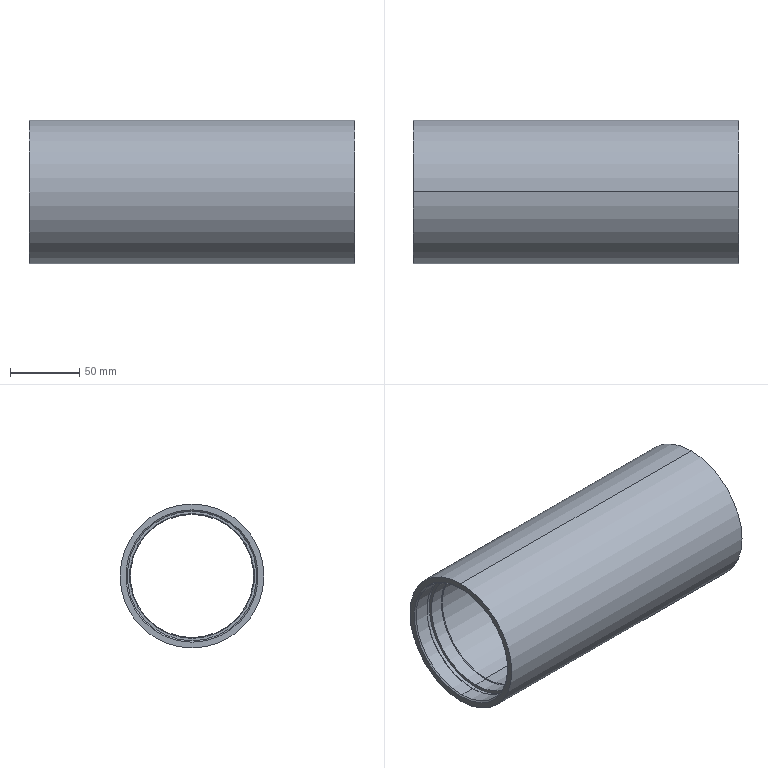Part | SolidWorks | features Chamfer 2, Revolution 1 | 1 solid | 30 faces | box 235 x 103.8 x 103.8 mm | volume 503241 mm3 | cylinder 16 | cone 8 | plane 6 | commonest cylinder face diameters 90 x4 93.5 x4 94.5 x4 89 x2 103.8 x2
STEP:
#1=CARTESIAN_POINT('',(25.5,0.,-44.5));
#2=VERTEX_POINT('',#1);
#3=CARTESIAN_POINT('',(25.5,0.,44.5));
#4=VERTEX_POINT('',#3);
#5=CARTESIAN_POINT('',(25.5,0.,0.));
#6=DIRECTION('',(-1.,0.,0.));
#7=DIRECTION('',(0.,0.,-1.));
#8=AXIS2_PLACEMENT_3D('',#5,#6,#7);
#9=CIRCLE('',#8,44.5);
#10=EDGE_CURVE('',#2,#4,#9,.T.);
#11=ORIENTED_EDGE('',*,*,#10,.F.);
#12=CARTESIAN_POINT('',(25.,0.,-45.));
#13=VERTEX_POINT('',#12);
#14=CARTESIAN_POINT('',(25.5,0.,-44.5));
#15=DIRECTION('',(-0.7071,0.,-0.7071));
#16=VECTOR('',#15,1000.);
#17=LINE('',#14,#16);
#18=EDGE_CURVE('',#2,#13,#17,.T.);
#19=ORIENTED_EDGE('',*,*,#18,.T.);
#20=CARTESIAN_POINT('',(25.,0.,45.));
#21=VERTEX_POINT('',#20);
#22=CARTESIAN_POINT('',(25.,0.,0.));
#23=DIRECTION('',(-1.,0.,0.));
#24=DIRECTION('',(0.,0.,1.));
#25=AXIS2_PLACEMENT_3D('',#22,#23,#24);
#26=CIRCLE('',#25,45.);
#27=EDGE_CURVE('',#13,#21,#26,.T.);
#28=ORIENTED_EDGE('',*,*,#27,.T.);
#29=CARTESIAN_POINT('',(25.5,0.,44.5));
#30=DIRECTION('',(-0.7071,0.,0.7071));
#31=VECTOR('',#30,1000.);
#32=LINE('',#29,#31);
#33=EDGE_CURVE('',#4,#21,#32,.T.);
#34=ORIENTED_EDGE('',*,*,#33,.F.);
#35=EDGE_LOOP('',(#11,#19,#28,#34));
#36=FACE_OUTER_BOUND('',#35,.T.);
#37=CARTESIAN_POINT('',(25.5,0.,0.));
#38=DIRECTION('',(-1.,0.,0.));
#39=DIRECTION('',(0.,0.,1.));
#40=AXIS2_PLACEMENT_3D('',#37,#38,#39);
#41=CONICAL_SURFACE('',#40,44.5,0.7854);
#42=ADVANCED_FACE('',(#36),#41,.F.);
#43=CARTESIAN_POINT('',(209.5,0.,44.5));
#44=VERTEX_POINT('',#43);
#45=CARTESIAN_POINT('',(209.5,0.,-44.5));
#46=VERTEX_POINT('',#45);
#47=CARTESIAN_POINT('',(209.5,0.,0.));
#48=DIRECTION('',(1.,0.,0.));
#49=DIRECTION('',(0.,0.,1.));
#50=AXIS2_PLACEMENT_3D('',#47,#48,#49);
#51=CIRCLE('',#50,44.5);
#52=EDGE_CURVE('',#44,#46,#51,.T.);
#53=ORIENTED_EDGE('',*,*,#52,.F.);
#54=CARTESIAN_POINT('',(210.,0.,45.));
#55=VERTEX_POINT('',#54);
#56=CARTESIAN_POINT('',(210.,0.,45.));
#57=DIRECTION('',(0.7071,0.,0.7071));
#58=VECTOR('',#57,1000.);
#59=LINE('',#56,#58);
#60=EDGE_CURVE('',#44,#55,#59,.T.);
#61=ORIENTED_EDGE('',*,*,#60,.T.);
#62=CARTESIAN_POINT('',(210.,0.,-45.));
#63=VERTEX_POINT('',#62);
#64=CARTESIAN_POINT('',(210.,0.,0.));
#65=DIRECTION('',(-1.,0.,0.));
#66=DIRECTION('',(0.,0.,1.));
#67=AXIS2_PLACEMENT_3D('',#64,#65,#66);
#68=CIRCLE('',#67,45.);
#69=EDGE_CURVE('',#63,#55,#68,.T.);
#70=ORIENTED_EDGE('',*,*,#69,.F.);
#71=CARTESIAN_POINT('',(210.,0.,-45.));
#72=DIRECTION('',(0.7071,0.,-0.7071));
#73=VECTOR('',#72,1000.);
#74=LINE('',#71,#73);
#75=EDGE_CURVE('',#46,#63,#74,.T.);
#76=ORIENTED_EDGE('',*,*,#75,.F.);
#77=EDGE_LOOP('',(#53,#61,#70,#76));
#78=FACE_OUTER_BOUND('',#77,.T.);
#79=CARTESIAN_POINT('',(210.,0.,0.));
#80=DIRECTION('',(1.,0.,0.));
#81=DIRECTION('',(0.,0.,-1.));
#82=AXIS2_PLACEMENT_3D('',#79,#80,#81);
#83=CONICAL_SURFACE('',#82,45.,0.7854);
#84=ADVANCED_FACE('',(#78),#83,.F.);
#85=CARTESIAN_POINT('',(1.,0.,-46.75));
#86=VERTEX_POINT('',#85);
#87=CARTESIAN_POINT('',(1.,0.,46.75));
#88=VERTEX_POINT('',#87);
#89=CARTESIAN_POINT('',(1.,0.,0.));
#90=DIRECTION('',(-1.,0.,0.));
#91=DIRECTION('',(0.,0.,-1.));
#92=AXIS2_PLACEMENT_3D('',#89,#90,#91);
#93=CIRCLE('',#92,46.75);
#94=EDGE_CURVE('',#86,#88,#93,.T.);
#95=ORIENTED_EDGE('',*,*,#94,.F.);
#96=CARTESIAN_POINT('',(0.,0.,-47.75));
#97=VERTEX_POINT('',#96);
#98=CARTESIAN_POINT('',(1.,0.,-46.75));
#99=DIRECTION('',(-0.7071,0.,-0.7071));
#100=VECTOR('',#99,1000.);
#101=LINE('',#98,#100);
#102=EDGE_CURVE('',#86,#97,#101,.T.);
#103=ORIENTED_EDGE('',*,*,#102,.T.);
#104=CARTESIAN_POINT('',(0.,0.,47.75));
#105=VERTEX_POINT('',#104);
#106=CARTESIAN_POINT('',(0.,0.,0.));
#107=DIRECTION('',(1.,0.,0.));
#108=DIRECTION('',(0.,0.,-1.));
#109=AXIS2_PLACEMENT_3D('',#106,#107,#108);
#110=CIRCLE('',#109,47.75);
#111=EDGE_CURVE('',#105,#97,#110,.T.);
#112=ORIENTED_EDGE('',*,*,#111,.F.);
#113=CARTESIAN_POINT('',(1.,0.,46.75));
#114=DIRECTION('',(-0.7071,0.,0.7071));
#115=VECTOR('',#114,1000.);
#116=LINE('',#113,#115);
#117=EDGE_CURVE('',#88,#105,#116,.T.);
#118=ORIENTED_EDGE('',*,*,#117,.F.);
#119=EDGE_LOOP('',(#95,#103,#112,#118));
#120=FACE_OUTER_BOUND('',#119,.T.);
#121=CARTESIAN_POINT('',(1.,0.,0.));
#122=DIRECTION('',(-1.,0.,0.));
#123=DIRECTION('',(0.,0.,1.));
#124=AXIS2_PLACEMENT_3D('',#121,#122,#123);
#125=CONICAL_SURFACE('',#124,46.75,0.7854);
#126=ADVANCED_FACE('',(#120),#125,.F.);
#127=CARTESIAN_POINT('',(234.,0.,46.75));
#128=VERTEX_POINT('',#127);
#129=CARTESIAN_POINT('',(234.,0.,-46.75));
#130=VERTEX_POINT('',#129);
#131=CARTESIAN_POINT('',(234.,0.,0.));
#132=DIRECTION('',(1.,0.,0.));
#133=DIRECTION('',(0.,0.,1.));
#134=AXIS2_PLACEMENT_3D('',#131,#132,#133);
#135=CIRCLE('',#134,46.75);
#136=EDGE_CURVE('',#128,#130,#135,.T.);
#137=ORIENTED_EDGE('',*,*,#136,.F.);
#138=CARTESIAN_POINT('',(235.,0.,47.75));
#139=VERTEX_POINT('',#138);
#140=CARTESIAN_POINT('',(235.,0.,47.75));
#141=DIRECTION('',(0.7071,0.,0.7071));
#142=VECTOR('',#141,1000.);
#143=LINE('',#140,#142);
#144=EDGE_CURVE('',#128,#139,#143,.T.);
#145=ORIENTED_EDGE('',*,*,#144,.T.);
#146=CARTESIAN_POINT('',(235.,0.,-47.75));
#147=VERTEX_POINT('',#146);
#148=CARTESIAN_POINT('',(235.,0.,0.));
#149=DIRECTION('',(-1.,0.,0.));
#150=DIRECTION('',(0.,0.,1.));
#151=AXIS2_PLACEMENT_3D('',#148,#149,#150);
#152=CIRCLE('',#151,47.75);
#153=EDGE_CURVE('',#147,#139,#152,.T.);
#154=ORIENTED_EDGE('',*,*,#153,.F.);
#155=CARTESIAN_POINT('',(235.,0.,-47.75));
#156=DIRECTION('',(0.7071,0.,-0.7071));
#157=VECTOR('',#156,1000.);
#158=LINE('',#155,#157);
#159=EDGE_CURVE('',#130,#147,#158,.T.);
#160=ORIENTED_EDGE('',*,*,#159,.F.);
#161=EDGE_LOOP('',(#137,#145,#154,#160));
#162=FACE_OUTER_BOUND('',#161,.T.);
#163=CARTESIAN_POINT('',(235.,0.,0.));
#164=DIRECTION('',(1.,0.,0.));
#165=DIRECTION('',(0.,0.,-1.));
#166=AXIS2_PLACEMENT_3D('',#163,#164,#165);
#167=CONICAL_SURFACE('',#166,47.75,0.7854);
#168=ADVANCED_FACE('',(#162),#167,.F.);
#169=CARTESIAN_POINT('',(12.,0.,-46.75));
#170=VERTEX_POINT('',#169);
#171=CARTESIAN_POINT('',(12.,0.,46.75));
#172=VERTEX_POINT('',#171);
#173=CARTESIAN_POINT('',(12.,0.,0.));
#174=DIRECTION('',(-1.,0.,0.));
#175=DIRECTION('',(0.,0.,1.));
#176=AXIS2_PLACEMENT_3D('',#173,#174,#175);
#177=CIRCLE('',#176,46.75);
#178=EDGE_CURVE('',#170,#172,#177,.T.);
#179=ORIENTED_EDGE('',*,*,#178,.F.);
#180=CARTESIAN_POINT('',(0.,0.,-46.75));
#181=DIRECTION('',(-1.,0.,0.));
#182=VECTOR('',#181,1000.);
#183=LINE('',#180,#182);
#184=EDGE_CURVE('',#170,#86,#183,.T.);
#185=ORIENTED_EDGE('',*,*,#184,.T.);
#186=ORIENTED_EDGE('',*,*,#94,.T.);
#187=CARTESIAN_POINT('',(0.,0.,46.75));
#188=DIRECTION('',(-1.,0.,0.));
#189=VECTOR('',#188,1000.);
#190=LINE('',#187,#189);
#191=EDGE_CURVE('',#172,#88,#190,.T.);
#192=ORIENTED_EDGE('',*,*,#191,.F.);
#193=EDGE_LOOP('',(#179,#185,#186,#192));
#194=FACE_OUTER_BOUND('',#193,.T.);
#195=CARTESIAN_POINT('',(0.,0.,0.));
#196=DIRECTION('',(-1.,0.,0.));
#197=DIRECTION('',(0.,0.,1.));
#198=AXIS2_PLACEMENT_3D('',#195,#196,#197);
#199=CYLINDRICAL_SURFACE('',#198,46.75);
#200=ADVANCED_FACE('',(#194),#199,.F.);
#201=CARTESIAN_POINT('',(15.,0.,-47.25));
#202=VERTEX_POINT('',#201);
#203=CARTESIAN_POINT('',(15.,0.,47.25));
#204=VERTEX_POINT('',#203);
#205=CARTESIAN_POINT('',(15.,0.,0.));
#206=DIRECTION('',(-1.,0.,0.));
#207=DIRECTION('',(0.,0.,1.));
#208=AXIS2_PLACEMENT_3D('',#205,#206,#207);
#209=CIRCLE('',#208,47.25);
#210=EDGE_CURVE('',#202,#204,#209,.T.);
#211=ORIENTED_EDGE('',*,*,#210,.F.);
#212=CARTESIAN_POINT('',(12.,0.,-47.25));
#213=VERTEX_POINT('',#212);
#214=CARTESIAN_POINT('',(0.,0.,-47.25));
#215=DIRECTION('',(-1.,0.,0.));
#216=VECTOR('',#215,1000.);
#217=LINE('',#214,#216);
#218=EDGE_CURVE('',#202,#213,#217,.T.);
#219=ORIENTED_EDGE('',*,*,#218,.T.);
#220=CARTESIAN_POINT('',(12.,0.,47.25));
#221=VERTEX_POINT('',#220);
#222=CARTESIAN_POINT('',(12.,0.,0.));
#223=DIRECTION('',(-1.,0.,0.));
#224=DIRECTION('',(0.,0.,1.));
#225=AXIS2_PLACEMENT_3D('',#222,#223,#224);
#226=CIRCLE('',#225,47.25);
#227=EDGE_CURVE('',#213,#221,#226,.T.);
#228=ORIENTED_EDGE('',*,*,#227,.T.);
#229=CARTESIAN_POINT('',(0.,0.,47.25));
#230=DIRECTION('',(-1.,0.,0.));
#231=VECTOR('',#230,1000.);
#232=LINE('',#229,#231);
#233=EDGE_CURVE('',#204,#221,#232,.T.);
#234=ORIENTED_EDGE('',*,*,#233,.F.);
#235=EDGE_LOOP('',(#211,#219,#228,#234));
#236=FACE_OUTER_BOUND('',#235,.T.);
#237=CARTESIAN_POINT('',(0.,0.,0.));
#238=DIRECTION('',(-1.,0.,0.));
#239=DIRECTION('',(0.,0.,1.));
#240=AXIS2_PLACEMENT_3D('',#237,#238,#239);
#241=CYLINDRICAL_SURFACE('',#240,47.25);
#242=ADVANCED_FACE('',(#236),#241,.F.);
#243=ORIENTED_EDGE('',*,*,#27,.F.);
#244=CARTESIAN_POINT('',(15.,0.,-45.));
#245=VERTEX_POINT('',#244);
#246=CARTESIAN_POINT('',(0.,0.,-45.));
#247=DIRECTION('',(-1.,0.,0.));
#248=VECTOR('',#247,1000.);
#249=LINE('',#246,#248);
#250=EDGE_CURVE('',#13,#245,#249,.T.);
#251=ORIENTED_EDGE('',*,*,#250,.T.);
#252=CARTESIAN_POINT('',(15.,0.,45.));
#253=VERTEX_POINT('',#252);
#254=CARTESIAN_POINT('',(15.,0.,0.));
#255=DIRECTION('',(-1.,0.,0.));
#256=DIRECTION('',(0.,0.,1.));
#257=AXIS2_PLACEMENT_3D('',#254,#255,#256);
#258=CIRCLE('',#257,45.);
#259=EDGE_CURVE('',#245,#253,#258,.T.);
#260=ORIENTED_EDGE('',*,*,#259,.T.);
#261=CARTESIAN_POINT('',(0.,0.,45.));
#262=DIRECTION('',(-1.,0.,0.));
#263=VECTOR('',#262,1000.);
#264=LINE('',#261,#263);
#265=EDGE_CURVE('',#21,#253,#264,.T.);
#266=ORIENTED_EDGE('',*,*,#265,.F.);
#267=EDGE_LOOP('',(#243,#251,#260,#266));
#268=FACE_OUTER_BOUND('',#267,.T.);
#269=CARTESIAN_POINT('',(0.,0.,0.));
#270=DIRECTION('',(-1.,0.,0.));
#271=DIRECTION('',(0.,0.,1.));
#272=AXIS2_PLACEMENT_3D('',#269,#270,#271);
#273=CYLINDRICAL_SURFACE('',#272,45.);
#274=ADVANCED_FACE('',(#268),#273,.F.);
#275=ORIENTED_EDGE('',*,*,#52,.T.);
#276=CARTESIAN_POINT('',(0.,0.,-44.5));
#277=DIRECTION('',(-1.,0.,0.));
#278=VECTOR('',#277,1000.);
#279=LINE('',#276,#278);
#280=EDGE_CURVE('',#46,#2,#279,.T.);
#281=ORIENTED_EDGE('',*,*,#280,.T.);
#282=ORIENTED_EDGE('',*,*,#10,.T.);
#283=CARTESIAN_POINT('',(0.,0.,44.5));
#284=DIRECTION('',(-1.,0.,0.));
#285=VECTOR('',#284,1000.);
#286=LINE('',#283,#285);
#287=EDGE_CURVE('',#44,#4,#286,.T.);
#288=ORIENTED_EDGE('',*,*,#287,.F.);
#289=EDGE_LOOP('',(#275,#281,#282,#288));
#290=FACE_OUTER_BOUND('',#289,.T.);
#291=CARTESIAN_POINT('',(0.,0.,0.));
#292=DIRECTION('',(-1.,0.,0.));
#293=DIRECTION('',(0.,0.,1.));
#294=AXIS2_PLACEMENT_3D('',#291,#292,#293);
#295=CYLINDRICAL_SURFACE('',#294,44.5);
#296=ADVANCED_FACE('',(#290),#295,.F.);
#297=CARTESIAN_POINT('',(220.,0.,-45.));
#298=VERTEX_POINT('',#297);
#299=CARTESIAN_POINT('',(220.,0.,45.));
#300=VERTEX_POINT('',#299);
#301=CARTESIAN_POINT('',(220.,0.,0.));
#302=DIRECTION('',(-1.,0.,0.));
#303=DIRECTION('',(0.,0.,1.));
#304=AXIS2_PLACEMENT_3D('',#301,#302,#303);
#305=CIRCLE('',#304,45.);
#306=EDGE_CURVE('',#298,#300,#305,.T.);
#307=ORIENTED_EDGE('',*,*,#306,.F.);
#308=CARTESIAN_POINT('',(0.,0.,-45.));
#309=DIRECTION('',(-1.,0.,0.));
#310=VECTOR('',#309,1000.);
#311=LINE('',#308,#310);
#312=EDGE_CURVE('',#298,#63,#311,.T.);
#313=ORIENTED_EDGE('',*,*,#312,.T.);
#314=ORIENTED_EDGE('',*,*,#69,.T.);
#315=CARTESIAN_POINT('',(0.,0.,45.));
#316=DIRECTION('',(-1.,0.,0.));
#317=VECTOR('',#316,1000.);
#318=LINE('',#315,#317);
#319=EDGE_CURVE('',#300,#55,#318,.T.);
#320=ORIENTED_EDGE('',*,*,#319,.F.);
#321=EDGE_LOOP('',(#307,#313,#314,#320));
#322=FACE_OUTER_BOUND('',#321,.T.);
#323=CARTESIAN_POINT('',(0.,0.,0.));
#324=DIRECTION('',(-1.,0.,0.));
#325=DIRECTION('',(0.,0.,1.));
#326=AXIS2_PLACEMENT_3D('',#323,#324,#325);
#327=CYLINDRICAL_SURFACE('',#326,45.);
#328=ADVANCED_FACE('',(#322),#327,.F.);
#329=CARTESIAN_POINT('',(223.,0.,-47.25));
#330=VERTEX_POINT('',#329);
#331=CARTESIAN_POINT('',(223.,0.,47.25));
#332=VERTEX_POINT('',#331);
#333=CARTESIAN_POINT('',(223.,0.,0.));
#334=DIRECTION('',(-1.,0.,0.));
#335=DIRECTION('',(0.,0.,1.));
#336=AXIS2_PLACEMENT_3D('',#333,#334,#335);
#337=CIRCLE('',#336,47.25);
#338=EDGE_CURVE('',#330,#332,#337,.T.);
#339=ORIENTED_EDGE('',*,*,#338,.F.);
#340=CARTESIAN_POINT('',(220.,0.,-47.25));
#341=VERTEX_POINT('',#340);
#342=CARTESIAN_POINT('',(0.,0.,-47.25));
#343=DIRECTION('',(-1.,0.,0.));
#344=VECTOR('',#343,1000.);
#345=LINE('',#342,#344);
#346=EDGE_CURVE('',#330,#341,#345,.T.);
#347=ORIENTED_EDGE('',*,*,#346,.T.);
#348=CARTESIAN_POINT('',(220.,0.,47.25));
#349=VERTEX_POINT('',#348);
#350=CARTESIAN_POINT('',(220.,0.,0.));
#351=DIRECTION('',(-1.,0.,0.));
#352=DIRECTION('',(0.,0.,1.));
#353=AXIS2_PLACEMENT_3D('',#350,#351,#352);
#354=CIRCLE('',#353,47.25);
#355=EDGE_CURVE('',#341,#349,#354,.T.);
#356=ORIENTED_EDGE('',*,*,#355,.T.);
#357=CARTESIAN_POINT('',(0.,0.,47.25));
#358=DIRECTION('',(-1.,0.,0.));
#359=VECTOR('',#358,1000.);
#360=LINE('',#357,#359);
#361=EDGE_CURVE('',#332,#349,#360,.T.);
#362=ORIENTED_EDGE('',*,*,#361,.F.);
#363=EDGE_LOOP('',(#339,#347,#356,#362));
#364=FACE_OUTER_BOUND('',#363,.T.);
#365=CARTESIAN_POINT('',(0.,0.,0.));
#366=DIRECTION('',(-1.,0.,0.));
#367=DIRECTION('',(0.,0.,1.));
#368=AXIS2_PLACEMENT_3D('',#365,#366,#367);
#369=CYLINDRICAL_SURFACE('',#368,47.25);
#370=ADVANCED_FACE('',(#364),#369,.F.);
#371=ORIENTED_EDGE('',*,*,#136,.T.);
#372=CARTESIAN_POINT('',(223.,0.,-46.75));
#373=VERTEX_POINT('',#372);
#374=CARTESIAN_POINT('',(0.,0.,-46.75));
#375=DIRECTION('',(-1.,0.,0.));
#376=VECTOR('',#375,1000.);
#377=LINE('',#374,#376);
#378=EDGE_CURVE('',#130,#373,#377,.T.);
#379=ORIENTED_EDGE('',*,*,#378,.T.);
#380=CARTESIAN_POINT('',(223.,0.,46.75));
#381=VERTEX_POINT('',#380);
#382=CARTESIAN_POINT('',(223.,0.,0.));
#383=DIRECTION('',(-1.,0.,0.));
#384=DIRECTION('',(0.,0.,1.));
#385=AXIS2_PLACEMENT_3D('',#382,#383,#384);
#386=CIRCLE('',#385,46.75);
#387=EDGE_CURVE('',#373,#381,#386,.T.);
#388=ORIENTED_EDGE('',*,*,#387,.T.);
#389=CARTESIAN_POINT('',(0.,0.,46.75));
#390=DIRECTION('',(-1.,0.,0.));
#391=VECTOR('',#390,1000.);
#392=LINE('',#389,#391);
#393=EDGE_CURVE('',#128,#381,#392,.T.);
#394=ORIENTED_EDGE('',*,*,#393,.F.);
#395=EDGE_LOOP('',(#371,#379,#388,#394));
#396=FACE_OUTER_BOUND('',#395,.T.);
#397=CARTESIAN_POINT('',(0.,0.,0.));
#398=DIRECTION('',(-1.,0.,0.));
#399=DIRECTION('',(0.,0.,1.));
#400=AXIS2_PLACEMENT_3D('',#397,#398,#399);
#401=CYLINDRICAL_SURFACE('',#400,46.75);
#402=ADVANCED_FACE('',(#396),#401,.F.);
#403=CARTESIAN_POINT('',(235.,0.,51.9));
#404=VERTEX_POINT('',#403);
#405=CARTESIAN_POINT('',(235.,0.,-51.9));
#406=VERTEX_POINT('',#405);
#407=CARTESIAN_POINT('',(235.,0.,0.));
#408=DIRECTION('',(-1.,0.,0.));
#409=DIRECTION('',(0.,0.,1.));
#410=AXIS2_PLACEMENT_3D('',#407,#408,#409);
#411=CIRCLE('',#410,51.9);
#412=EDGE_CURVE('',#404,#406,#411,.T.);
#413=ORIENTED_EDGE('',*,*,#412,.T.);
#414=CARTESIAN_POINT('',(0.,0.,-51.9));
#415=VERTEX_POINT('',#414);
#416=CARTESIAN_POINT('',(0.,0.,-51.9));
#417=DIRECTION('',(-1.,0.,0.));
#418=VECTOR('',#417,1000.);
#419=LINE('',#416,#418);
#420=EDGE_CURVE('',#406,#415,#419,.T.);
#421=ORIENTED_EDGE('',*,*,#420,.T.);
#422=CARTESIAN_POINT('',(0.,0.,51.9));
#423=VERTEX_POINT('',#422);
#424=CARTESIAN_POINT('',(0.,0.,0.));
#425=DIRECTION('',(-1.,0.,0.));
#426=DIRECTION('',(0.,0.,1.));
#427=AXIS2_PLACEMENT_3D('',#424,#425,#426);
#428=CIRCLE('',#427,51.9);
#429=EDGE_CURVE('',#423,#415,#428,.T.);
#430=ORIENTED_EDGE('',*,*,#429,.F.);
#431=CARTESIAN_POINT('',(0.,0.,51.9));
#432=DIRECTION('',(-1.,0.,0.));
#433=VECTOR('',#432,1000.);
#434=LINE('',#431,#433);
#435=EDGE_CURVE('',#404,#423,#434,.T.);
#436=ORIENTED_EDGE('',*,*,#435,.F.);
#437=EDGE_LOOP('',(#413,#421,#430,#436));
#438=FACE_OUTER_BOUND('',#437,.T.);
#439=CARTESIAN_POINT('',(0.,0.,0.));
#440=DIRECTION('',(-1.,0.,0.));
#441=DIRECTION('',(0.,0.,1.));
#442=AXIS2_PLACEMENT_3D('',#439,#440,#441);
#443=CYLINDRICAL_SURFACE('',#442,51.9);
#444=ADVANCED_FACE('',(#438),#443,.T.);
#445=ORIENTED_EDGE('',*,*,#111,.T.);
#446=CARTESIAN_POINT('',(0.,0.,0.));
#447=DIRECTION('',(1.,0.,0.));
#448=DIRECTION('',(0.,0.,-1.));
#449=AXIS2_PLACEMENT_3D('',#446,#447,#448);
#450=CIRCLE('',#449,47.75);
#451=EDGE_CURVE('',#97,#105,#450,.T.);
#452=ORIENTED_EDGE('',*,*,#451,.T.);
#453=EDGE_LOOP('',(#445,#452));
#454=FACE_BOUND('',#453,.T.);
#455=ORIENTED_EDGE('',*,*,#429,.T.);
#456=CARTESIAN_POINT('',(0.,0.,0.));
#457=DIRECTION('',(-1.,0.,0.));
#458=DIRECTION('',(0.,0.,1.));
#459=AXIS2_PLACEMENT_3D('',#456,#457,#458);
#460=CIRCLE('',#459,51.9);
#461=EDGE_CURVE('',#415,#423,#460,.T.);
#462=ORIENTED_EDGE('',*,*,#461,.T.);
#463=EDGE_LOOP('',(#455,#462));
#464=FACE_OUTER_BOUND('',#463,.T.);
#465=CARTESIAN_POINT('',(0.,0.,-46.75));
#466=DIRECTION('',(1.,0.,0.));
#467=DIRECTION('',(0.,0.,-1.));
#468=AXIS2_PLACEMENT_3D('',#465,#466,#467);
#469=PLANE('',#468);
#470=ADVANCED_FACE('',(#454,#464),#469,.F.);
#471=ORIENTED_EDGE('',*,*,#420,.F.);
#472=CARTESIAN_POINT('',(235.,0.,0.));
#473=DIRECTION('',(-1.,0.,0.));
#474=DIRECTION('',(0.,0.,1.));
#475=AXIS2_PLACEMENT_3D('',#472,#473,#474);
#476=CIRCLE('',#475,51.9);
#477=EDGE_CURVE('',#406,#404,#476,.T.);
#478=ORIENTED_EDGE('',*,*,#477,.T.);
#479=ORIENTED_EDGE('',*,*,#435,.T.);
#480=ORIENTED_EDGE('',*,*,#461,.F.);
#481=EDGE_LOOP('',(#471,#478,#479,#480));
#482=FACE_OUTER_BOUND('',#481,.T.);
#483=CARTESIAN_POINT('',(0.,0.,0.));
#484=DIRECTION('',(-1.,0.,0.));
#485=DIRECTION('',(0.,0.,1.));
#486=AXIS2_PLACEMENT_3D('',#483,#484,#485);
#487=CYLINDRICAL_SURFACE('',#486,51.9);
#488=ADVANCED_FACE('',(#482),#487,.T.);
#489=ORIENTED_EDGE('',*,*,#153,.T.);
#490=CARTESIAN_POINT('',(235.,0.,0.));
#491=DIRECTION('',(-1.,0.,0.));
#492=DIRECTION('',(0.,0.,1.));
#493=AXIS2_PLACEMENT_3D('',#490,#491,#492);
#494=CIRCLE('',#493,47.75);
#495=EDGE_CURVE('',#139,#147,#494,.T.);
#496=ORIENTED_EDGE('',*,*,#495,.T.);
#497=EDGE_LOOP('',(#489,#496));
#498=FACE_BOUND('',#497,.T.);
#499=ORIENTED_EDGE('',*,*,#412,.F.);
#500=ORIENTED_EDGE('',*,*,#477,.F.);
#501=EDGE_LOOP('',(#499,#500));
#502=FACE_OUTER_BOUND('',#501,.T.);
#503=CARTESIAN_POINT('',(235.,0.,-46.75));
#504=DIRECTION('',(-1.,0.,0.));
#505=DIRECTION('',(0.,0.,1.));
#506=AXIS2_PLACEMENT_3D('',#503,#504,#505);
#507=PLANE('',#506);
#508=ADVANCED_FACE('',(#498,#502),#507,.F.);
#509=ORIENTED_EDGE('',*,*,#378,.F.);
#510=CARTESIAN_POINT('',(234.,0.,0.));
#511=DIRECTION('',(1.,0.,0.));
#512=DIRECTION('',(0.,0.,1.));
#513=AXIS2_PLACEMENT_3D('',#510,#511,#512);
#514=CIRCLE('',#513,46.75);
#515=EDGE_CURVE('',#130,#128,#514,.T.);
#516=ORIENTED_EDGE('',*,*,#515,.T.);
#517=ORIENTED_EDGE('',*,*,#393,.T.);
#518=CARTESIAN_POINT('',(223.,0.,0.));
#519=DIRECTION('',(-1.,0.,0.));
#520=DIRECTION('',(0.,0.,1.));
#521=AXIS2_PLACEMENT_3D('',#518,#519,#520);
#522=CIRCLE('',#521,46.75);
#523=EDGE_CURVE('',#381,#373,#522,.T.);
#524=ORIENTED_EDGE('',*,*,#523,.T.);
#525=EDGE_LOOP('',(#509,#516,#517,#524));
#526=FACE_OUTER_BOUND('',#525,.T.);
#527=CARTESIAN_POINT('',(0.,0.,0.));
#528=DIRECTION('',(-1.,0.,0.));
#529=DIRECTION('',(0.,0.,1.));
#530=AXIS2_PLACEMENT_3D('',#527,#528,#529);
#531=CYLINDRICAL_SURFACE('',#530,46.75);
#532=ADVANCED_FACE('',(#526),#531,.F.);
#533=ORIENTED_EDGE('',*,*,#523,.F.);
#534=ORIENTED_EDGE('',*,*,#387,.F.);
#535=EDGE_LOOP('',(#533,#534));
#536=FACE_BOUND('',#535,.T.);
#537=CARTESIAN_POINT('',(223.,0.,0.));
#538=DIRECTION('',(-1.,0.,0.));
#539=DIRECTION('',(0.,0.,1.));
#540=AXIS2_PLACEMENT_3D('',#537,#538,#539);
#541=CIRCLE('',#540,47.25);
#542=EDGE_CURVE('',#332,#330,#541,.T.);
#543=ORIENTED_EDGE('',*,*,#542,.T.);
#544=ORIENTED_EDGE('',*,*,#338,.T.);
#545=EDGE_LOOP('',(#543,#544));
#546=FACE_OUTER_BOUND('',#545,.T.);
#547=CARTESIAN_POINT('',(223.,0.,-46.75));
#548=DIRECTION('',(1.,0.,0.));
#549=DIRECTION('',(0.,0.,-1.));
#550=AXIS2_PLACEMENT_3D('',#547,#548,#549);
#551=PLANE('',#550);
#552=ADVANCED_FACE('',(#536,#546),#551,.F.);
#553=ORIENTED_EDGE('',*,*,#346,.F.);
#554=ORIENTED_EDGE('',*,*,#542,.F.);
#555=ORIENTED_EDGE('',*,*,#361,.T.);
#556=CARTESIAN_POINT('',(220.,0.,0.));
#557=DIRECTION('',(-1.,0.,0.));
#558=DIRECTION('',(0.,0.,1.));
#559=AXIS2_PLACEMENT_3D('',#556,#557,#558);
#560=CIRCLE('',#559,47.25);
#561=EDGE_CURVE('',#349,#341,#560,.T.);
#562=ORIENTED_EDGE('',*,*,#561,.T.);
#563=EDGE_LOOP('',(#553,#554,#555,#562));
#564=FACE_OUTER_BOUND('',#563,.T.);
#565=CARTESIAN_POINT('',(0.,0.,0.));
#566=DIRECTION('',(-1.,0.,0.));
#567=DIRECTION('',(0.,0.,1.));
#568=AXIS2_PLACEMENT_3D('',#565,#566,#567);
#569=CYLINDRICAL_SURFACE('',#568,47.25);
#570=ADVANCED_FACE('',(#564),#569,.F.);
#571=ORIENTED_EDGE('',*,*,#561,.F.);
#572=ORIENTED_EDGE('',*,*,#355,.F.);
#573=EDGE_LOOP('',(#571,#572));
#574=FACE_OUTER_BOUND('',#573,.T.);
#575=CARTESIAN_POINT('',(220.,0.,0.));
#576=DIRECTION('',(-1.,0.,0.));
#577=DIRECTION('',(0.,0.,1.));
#578=AXIS2_PLACEMENT_3D('',#575,#576,#577);
#579=CIRCLE('',#578,45.);
#580=EDGE_CURVE('',#300,#298,#579,.T.);
#581=ORIENTED_EDGE('',*,*,#580,.T.);
#582=ORIENTED_EDGE('',*,*,#306,.T.);
#583=EDGE_LOOP('',(#581,#582));
#584=FACE_BOUND('',#583,.T.);
#585=CARTESIAN_POINT('',(220.,0.,-47.25));
#586=DIRECTION('',(-1.,0.,0.));
#587=DIRECTION('',(0.,0.,1.));
#588=AXIS2_PLACEMENT_3D('',#585,#586,#587);
#589=PLANE('',#588);
#590=ADVANCED_FACE('',(#574,#584),#589,.F.);
#591=ORIENTED_EDGE('',*,*,#312,.F.);
#592=ORIENTED_EDGE('',*,*,#580,.F.);
#593=ORIENTED_EDGE('',*,*,#319,.T.);
#594=CARTESIAN_POINT('',(210.,0.,0.));
#595=DIRECTION('',(-1.,0.,0.));
#596=DIRECTION('',(0.,0.,1.));
#597=AXIS2_PLACEMENT_3D('',#594,#595,#596);
#598=CIRCLE('',#597,45.);
#599=EDGE_CURVE('',#55,#63,#598,.T.);
#600=ORIENTED_EDGE('',*,*,#599,.T.);
#601=EDGE_LOOP('',(#591,#592,#593,#600));
#602=FACE_OUTER_BOUND('',#601,.T.);
#603=CARTESIAN_POINT('',(0.,0.,0.));
#604=DIRECTION('',(-1.,0.,0.));
#605=DIRECTION('',(0.,0.,1.));
#606=AXIS2_PLACEMENT_3D('',#603,#604,#605);
#607=CYLINDRICAL_SURFACE('',#606,45.);
#608=ADVANCED_FACE('',(#602),#607,.F.);
#609=ORIENTED_EDGE('',*,*,#280,.F.);
#610=CARTESIAN_POINT('',(209.5,0.,0.));
#611=DIRECTION('',(1.,0.,0.));
#612=DIRECTION('',(0.,0.,1.));
#613=AXIS2_PLACEMENT_3D('',#610,#611,#612);
#614=CIRCLE('',#613,44.5);
#615=EDGE_CURVE('',#46,#44,#614,.T.);
#616=ORIENTED_EDGE('',*,*,#615,.T.);
#617=ORIENTED_EDGE('',*,*,#287,.T.);
#618=CARTESIAN_POINT('',(25.5,0.,0.));
#619=DIRECTION('',(-1.,0.,0.));
#620=DIRECTION('',(0.,0.,-1.));
#621=AXIS2_PLACEMENT_3D('',#618,#619,#620);
#622=CIRCLE('',#621,44.5);
#623=EDGE_CURVE('',#4,#2,#622,.T.);
#624=ORIENTED_EDGE('',*,*,#623,.T.);
#625=EDGE_LOOP('',(#609,#616,#617,#624));
#626=FACE_OUTER_BOUND('',#625,.T.);
#627=CARTESIAN_POINT('',(0.,0.,0.));
#628=DIRECTION('',(-1.,0.,0.));
#629=DIRECTION('',(0.,0.,1.));
#630=AXIS2_PLACEMENT_3D('',#627,#628,#629);
#631=CYLINDRICAL_SURFACE('',#630,44.5);
#632=ADVANCED_FACE('',(#626),#631,.F.);
#633=ORIENTED_EDGE('',*,*,#250,.F.);
#634=CARTESIAN_POINT('',(25.,0.,0.));
#635=DIRECTION('',(-1.,0.,0.));
#636=DIRECTION('',(0.,0.,1.));
#637=AXIS2_PLACEMENT_3D('',#634,#635,#636);
#638=CIRCLE('',#637,45.);
#639=EDGE_CURVE('',#21,#13,#638,.T.);
#640=ORIENTED_EDGE('',*,*,#639,.F.);
#641=ORIENTED_EDGE('',*,*,#265,.T.);
#642=CARTESIAN_POINT('',(15.,0.,0.));
#643=DIRECTION('',(-1.,0.,0.));
#644=DIRECTION('',(0.,0.,1.));
#645=AXIS2_PLACEMENT_3D('',#642,#643,#644);
#646=CIRCLE('',#645,45.);
#647=EDGE_CURVE('',#253,#245,#646,.T.);
#648=ORIENTED_EDGE('',*,*,#647,.T.);
#649=EDGE_LOOP('',(#633,#640,#641,#648));
#650=FACE_OUTER_BOUND('',#649,.T.);
#651=CARTESIAN_POINT('',(0.,0.,0.));
#652=DIRECTION('',(-1.,0.,0.));
#653=DIRECTION('',(0.,0.,1.));
#654=AXIS2_PLACEMENT_3D('',#651,#652,#653);
#655=CYLINDRICAL_SURFACE('',#654,45.);
#656=ADVANCED_FACE('',(#650),#655,.F.);
#657=ORIENTED_EDGE('',*,*,#647,.F.);
#658=ORIENTED_EDGE('',*,*,#259,.F.);
#659=EDGE_LOOP('',(#657,#658));
#660=FACE_BOUND('',#659,.T.);
#661=CARTESIAN_POINT('',(15.,0.,0.));
#662=DIRECTION('',(-1.,0.,0.));
#663=DIRECTION('',(0.,0.,1.));
#664=AXIS2_PLACEMENT_3D('',#661,#662,#663);
#665=CIRCLE('',#664,47.25);
#666=EDGE_CURVE('',#204,#202,#665,.T.);
#667=ORIENTED_EDGE('',*,*,#666,.T.);
#668=ORIENTED_EDGE('',*,*,#210,.T.);
#669=EDGE_LOOP('',(#667,#668));
#670=FACE_OUTER_BOUND('',#669,.T.);
#671=CARTESIAN_POINT('',(15.,0.,-47.25));
#672=DIRECTION('',(1.,0.,0.));
#673=DIRECTION('',(0.,0.,-1.));
#674=AXIS2_PLACEMENT_3D('',#671,#672,#673);
#675=PLANE('',#674);
#676=ADVANCED_FACE('',(#660,#670),#675,.F.);
#677=ORIENTED_EDGE('',*,*,#218,.F.);
#678=ORIENTED_EDGE('',*,*,#666,.F.);
#679=ORIENTED_EDGE('',*,*,#233,.T.);
#680=CARTESIAN_POINT('',(12.,0.,0.));
#681=DIRECTION('',(-1.,0.,0.));
#682=DIRECTION('',(0.,0.,1.));
#683=AXIS2_PLACEMENT_3D('',#680,#681,#682);
#684=CIRCLE('',#683,47.25);
#685=EDGE_CURVE('',#221,#213,#684,.T.);
#686=ORIENTED_EDGE('',*,*,#685,.T.);
#687=EDGE_LOOP('',(#677,#678,#679,#686));
#688=FACE_OUTER_BOUND('',#687,.T.);
#689=CARTESIAN_POINT('',(0.,0.,0.));
#690=DIRECTION('',(-1.,0.,0.));
#691=DIRECTION('',(0.,0.,1.));
#692=AXIS2_PLACEMENT_3D('',#689,#690,#691);
#693=CYLINDRICAL_SURFACE('',#692,47.25);
#694=ADVANCED_FACE('',(#688),#693,.F.);
#695=ORIENTED_EDGE('',*,*,#685,.F.);
#696=ORIENTED_EDGE('',*,*,#227,.F.);
#697=EDGE_LOOP('',(#695,#696));
#698=FACE_OUTER_BOUND('',#697,.T.);
#699=CARTESIAN_POINT('',(12.,0.,0.));
#700=DIRECTION('',(-1.,0.,0.));
#701=DIRECTION('',(0.,0.,1.));
#702=AXIS2_PLACEMENT_3D('',#699,#700,#701);
#703=CIRCLE('',#702,46.75);
#704=EDGE_CURVE('',#172,#170,#703,.T.);
#705=ORIENTED_EDGE('',*,*,#704,.T.);
#706=ORIENTED_EDGE('',*,*,#178,.T.);
#707=EDGE_LOOP('',(#705,#706));
#708=FACE_BOUND('',#707,.T.);
#709=CARTESIAN_POINT('',(12.,0.,-46.75));
#710=DIRECTION('',(-1.,0.,0.));
#711=DIRECTION('',(0.,0.,1.));
#712=AXIS2_PLACEMENT_3D('',#709,#710,#711);
#713=PLANE('',#712);
#714=ADVANCED_FACE('',(#698,#708),#713,.F.);
#715=ORIENTED_EDGE('',*,*,#184,.F.);
#716=ORIENTED_EDGE('',*,*,#704,.F.);
#717=ORIENTED_EDGE('',*,*,#191,.T.);
#718=CARTESIAN_POINT('',(1.,0.,0.));
#719=DIRECTION('',(-1.,0.,0.));
#720=DIRECTION('',(0.,0.,-1.));
#721=AXIS2_PLACEMENT_3D('',#718,#719,#720);
#722=CIRCLE('',#721,46.75);
#723=EDGE_CURVE('',#88,#86,#722,.T.);
#724=ORIENTED_EDGE('',*,*,#723,.T.);
#725=EDGE_LOOP('',(#715,#716,#717,#724));
#726=FACE_OUTER_BOUND('',#725,.T.);
#727=CARTESIAN_POINT('',(0.,0.,0.));
#728=DIRECTION('',(-1.,0.,0.));
#729=DIRECTION('',(0.,0.,1.));
#730=AXIS2_PLACEMENT_3D('',#727,#728,#729);
#731=CYLINDRICAL_SURFACE('',#730,46.75);
#732=ADVANCED_FACE('',(#726),#731,.F.);
#733=ORIENTED_EDGE('',*,*,#144,.F.);
#734=ORIENTED_EDGE('',*,*,#515,.F.);
#735=ORIENTED_EDGE('',*,*,#159,.T.);
#736=ORIENTED_EDGE('',*,*,#495,.F.);
#737=EDGE_LOOP('',(#733,#734,#735,#736));
#738=FACE_OUTER_BOUND('',#737,.T.);
#739=CARTESIAN_POINT('',(235.,0.,0.));
#740=DIRECTION('',(1.,0.,0.));
#741=DIRECTION('',(0.,0.,-1.));
#742=AXIS2_PLACEMENT_3D('',#739,#740,#741);
#743=CONICAL_SURFACE('',#742,47.75,0.7854);
#744=ADVANCED_FACE('',(#738),#743,.F.);
#745=ORIENTED_EDGE('',*,*,#102,.F.);
#746=ORIENTED_EDGE('',*,*,#723,.F.);
#747=ORIENTED_EDGE('',*,*,#117,.T.);
#748=ORIENTED_EDGE('',*,*,#451,.F.);
#749=EDGE_LOOP('',(#745,#746,#747,#748));
#750=FACE_OUTER_BOUND('',#749,.T.);
#751=CARTESIAN_POINT('',(1.,0.,0.));
#752=DIRECTION('',(-1.,0.,0.));
#753=DIRECTION('',(0.,0.,1.));
#754=AXIS2_PLACEMENT_3D('',#751,#752,#753);
#755=CONICAL_SURFACE('',#754,46.75,0.7854);
#756=ADVANCED_FACE('',(#750),#755,.F.);
#757=ORIENTED_EDGE('',*,*,#60,.F.);
#758=ORIENTED_EDGE('',*,*,#615,.F.);
#759=ORIENTED_EDGE('',*,*,#75,.T.);
#760=ORIENTED_EDGE('',*,*,#599,.F.);
#761=EDGE_LOOP('',(#757,#758,#759,#760));
#762=FACE_OUTER_BOUND('',#761,.T.);
#763=CARTESIAN_POINT('',(210.,0.,0.));
#764=DIRECTION('',(1.,0.,0.));
#765=DIRECTION('',(0.,0.,-1.));
#766=AXIS2_PLACEMENT_3D('',#763,#764,#765);
#767=CONICAL_SURFACE('',#766,45.,0.7854);
#768=ADVANCED_FACE('',(#762),#767,.F.);
#769=ORIENTED_EDGE('',*,*,#18,.F.);
#770=ORIENTED_EDGE('',*,*,#623,.F.);
#771=ORIENTED_EDGE('',*,*,#33,.T.);
#772=ORIENTED_EDGE('',*,*,#639,.T.);
#773=EDGE_LOOP('',(#769,#770,#771,#772));
#774=FACE_OUTER_BOUND('',#773,.T.);
#775=CARTESIAN_POINT('',(25.5,0.,0.));
#776=DIRECTION('',(-1.,0.,0.));
#777=DIRECTION('',(0.,0.,1.));
#778=AXIS2_PLACEMENT_3D('',#775,#776,#777);
#779=CONICAL_SURFACE('',#778,44.5,0.7854);
#780=ADVANCED_FACE('',(#774),#779,.F.);
#781=CLOSED_SHELL('',(#42,#84,#126,#168,#200,#242,#274,#296,#328,#370,#402,#444,#470,#488,#508,#532,#552,#570,#590,#608,#632,#656,#676,#694,#714,#732,#744,#756,#768,#780));
#782=MANIFOLD_SOLID_BREP('',#781);
#783=CARTESIAN_POINT('',(0.,0.,0.));
#784=DIRECTION('',(0.,0.,1.));
#785=DIRECTION('',(1.,0.,0.));
#786=AXIS2_PLACEMENT_3D('',#783,#784,#785);
#787=(LENGTH_UNIT()NAMED_UNIT(*)SI_UNIT(.MILLI.,.METRE.));
#788=UNCERTAINTY_MEASURE_WITH_UNIT(LENGTH_MEASURE(0.00001),#787,'','');
#789=(NAMED_UNIT(*)PLANE_ANGLE_UNIT()SI_UNIT($,.RADIAN.));
#790=(NAMED_UNIT(*)SI_UNIT($,.STERADIAN.)SOLID_ANGLE_UNIT());
#791=(GEOMETRIC_REPRESENTATION_CONTEXT(3)GLOBAL_UNCERTAINTY_ASSIGNED_CONTEXT((#788))GLOBAL_UNIT_ASSIGNED_CONTEXT((#787,#789,#790))REPRESENTATION_CONTEXT('',''));
#792=ADVANCED_BREP_SHAPE_REPRESENTATION('',(#782,#786),#791);